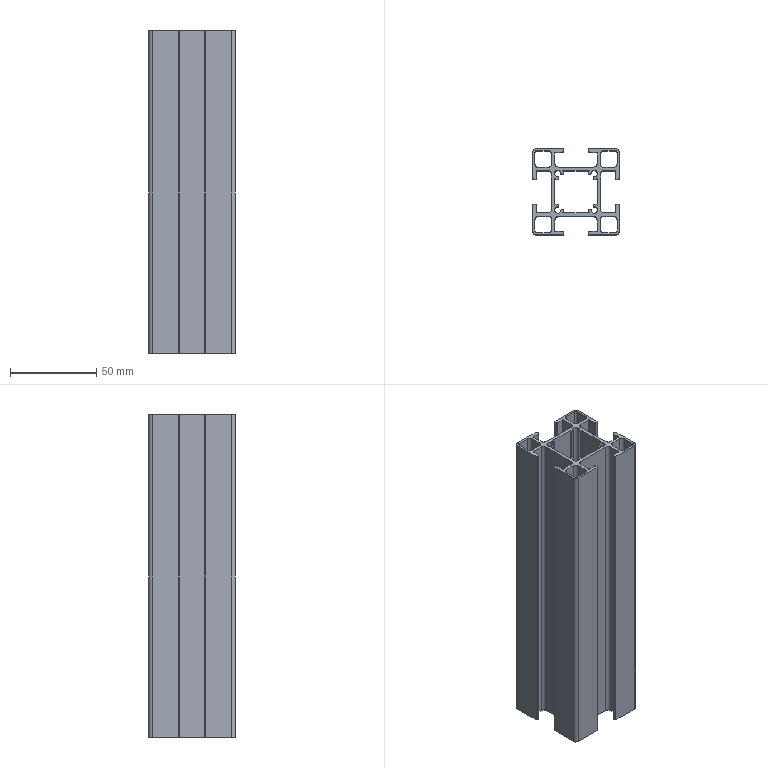Part | STEP file | 46A-00006CC11-187mm | 1 solid | 142 faces | box 50 x 50 x 187 mm | volume 109861 mm3 | cylinder 84 | plane 58 | commonest cylinder face diameters 1 x24 4 x24 1.5 x16 3.7 x8 6.7 x8 2 x4